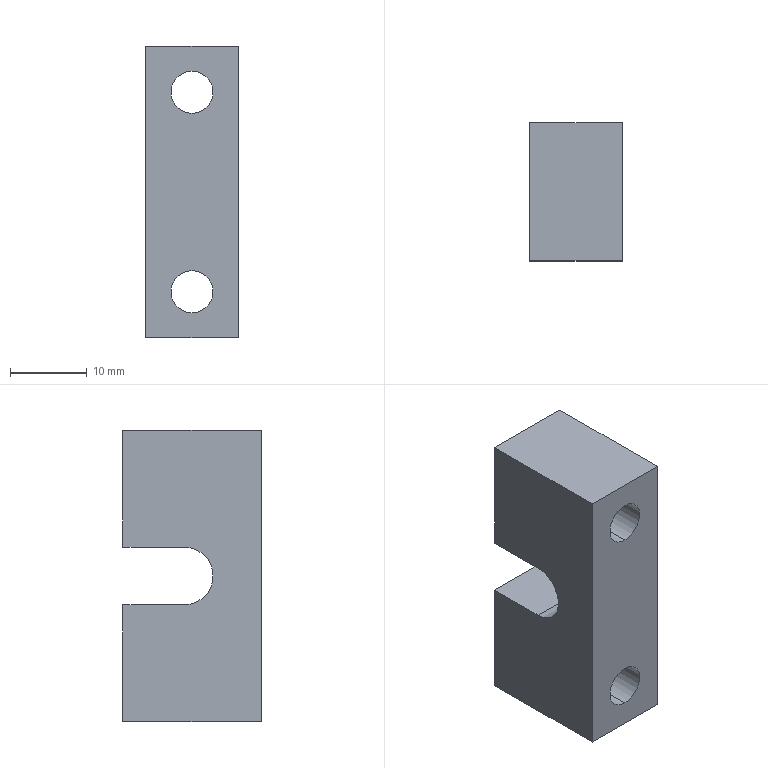Part | SolidWorks | features BaseBody 1 | 1 solid | 20 faces | box 12 x 18 x 38 mm | volume 5849 mm3 | plane 11 | cylinder 9 | commonest cylinder face diameters 5.5 x4 9.5 x4 7.5 x1
STEP:
#1=CARTESIAN_POINT('',(0.,12.5,8.25));
#2=VERTEX_POINT('',#1);
#3=CARTESIAN_POINT('',(0.,12.5,17.75));
#4=VERTEX_POINT('',#3);
#5=CARTESIAN_POINT('',(0.,12.5,13.));
#6=DIRECTION('',(0.,1.,0.));
#7=DIRECTION('',(0.,0.,1.));
#8=AXIS2_PLACEMENT_3D('',#5,#6,#7);
#9=CIRCLE('',#8,4.75);
#10=EDGE_CURVE('',#2,#4,#9,.T.);
#11=ORIENTED_EDGE('',*,*,#10,.F.);
#12=CARTESIAN_POINT('',(0.,18.,8.25));
#13=VERTEX_POINT('',#12);
#14=CARTESIAN_POINT('',(0.,18.,8.25));
#15=DIRECTION('',(0.,1.,0.));
#16=VECTOR('',#15,1000.);
#17=LINE('',#14,#16);
#18=EDGE_CURVE('',#2,#13,#17,.T.);
#19=ORIENTED_EDGE('',*,*,#18,.T.);
#20=CARTESIAN_POINT('',(0.,18.,17.75));
#21=VERTEX_POINT('',#20);
#22=CARTESIAN_POINT('',(0.,18.,13.));
#23=DIRECTION('',(0.,1.,0.));
#24=DIRECTION('',(0.,0.,1.));
#25=AXIS2_PLACEMENT_3D('',#22,#23,#24);
#26=CIRCLE('',#25,4.75);
#27=EDGE_CURVE('',#13,#21,#26,.T.);
#28=ORIENTED_EDGE('',*,*,#27,.T.);
#29=CARTESIAN_POINT('',(0.,18.,17.75));
#30=DIRECTION('',(0.,1.,0.));
#31=VECTOR('',#30,1000.);
#32=LINE('',#29,#31);
#33=EDGE_CURVE('',#4,#21,#32,.T.);
#34=ORIENTED_EDGE('',*,*,#33,.F.);
#35=EDGE_LOOP('',(#11,#19,#28,#34));
#36=FACE_OUTER_BOUND('',#35,.T.);
#37=CARTESIAN_POINT('',(0.,18.,13.));
#38=DIRECTION('',(0.,1.,0.));
#39=DIRECTION('',(0.,0.,1.));
#40=AXIS2_PLACEMENT_3D('',#37,#38,#39);
#41=CYLINDRICAL_SURFACE('',#40,4.75);
#42=ADVANCED_FACE('',(#36),#41,.F.);
#43=CARTESIAN_POINT('',(0.,12.5,-17.75));
#44=VERTEX_POINT('',#43);
#45=CARTESIAN_POINT('',(0.,12.5,-8.25));
#46=VERTEX_POINT('',#45);
#47=CARTESIAN_POINT('',(0.,12.5,-13.));
#48=DIRECTION('',(0.,1.,0.));
#49=DIRECTION('',(0.,0.,1.));
#50=AXIS2_PLACEMENT_3D('',#47,#48,#49);
#51=CIRCLE('',#50,4.75);
#52=EDGE_CURVE('',#44,#46,#51,.T.);
#53=ORIENTED_EDGE('',*,*,#52,.F.);
#54=CARTESIAN_POINT('',(0.,18.,-17.75));
#55=VERTEX_POINT('',#54);
#56=CARTESIAN_POINT('',(0.,18.,-17.75));
#57=DIRECTION('',(0.,1.,0.));
#58=VECTOR('',#57,1000.);
#59=LINE('',#56,#58);
#60=EDGE_CURVE('',#44,#55,#59,.T.);
#61=ORIENTED_EDGE('',*,*,#60,.T.);
#62=CARTESIAN_POINT('',(0.,18.,-8.25));
#63=VERTEX_POINT('',#62);
#64=CARTESIAN_POINT('',(0.,18.,-13.));
#65=DIRECTION('',(0.,1.,0.));
#66=DIRECTION('',(0.,0.,1.));
#67=AXIS2_PLACEMENT_3D('',#64,#65,#66);
#68=CIRCLE('',#67,4.75);
#69=EDGE_CURVE('',#55,#63,#68,.T.);
#70=ORIENTED_EDGE('',*,*,#69,.T.);
#71=CARTESIAN_POINT('',(0.,18.,-8.25));
#72=DIRECTION('',(0.,1.,0.));
#73=VECTOR('',#72,1000.);
#74=LINE('',#71,#73);
#75=EDGE_CURVE('',#46,#63,#74,.T.);
#76=ORIENTED_EDGE('',*,*,#75,.F.);
#77=EDGE_LOOP('',(#53,#61,#70,#76));
#78=FACE_OUTER_BOUND('',#77,.T.);
#79=CARTESIAN_POINT('',(0.,18.,-13.));
#80=DIRECTION('',(0.,1.,0.));
#81=DIRECTION('',(0.,0.,1.));
#82=AXIS2_PLACEMENT_3D('',#79,#80,#81);
#83=CYLINDRICAL_SURFACE('',#82,4.75);
#84=ADVANCED_FACE('',(#78),#83,.F.);
#85=CARTESIAN_POINT('',(0.,0.,-10.25));
#86=VERTEX_POINT('',#85);
#87=CARTESIAN_POINT('',(0.,0.,-15.75));
#88=VERTEX_POINT('',#87);
#89=CARTESIAN_POINT('',(0.,0.,-13.));
#90=DIRECTION('',(0.,-1.,0.));
#91=DIRECTION('',(0.,0.,1.));
#92=AXIS2_PLACEMENT_3D('',#89,#90,#91);
#93=CIRCLE('',#92,2.75);
#94=EDGE_CURVE('',#86,#88,#93,.T.);
#95=ORIENTED_EDGE('',*,*,#94,.T.);
#96=CARTESIAN_POINT('',(0.,12.5,-15.75));
#97=VERTEX_POINT('',#96);
#98=CARTESIAN_POINT('',(0.,18.,-15.75));
#99=DIRECTION('',(0.,1.,0.));
#100=VECTOR('',#99,1000.);
#101=LINE('',#98,#100);
#102=EDGE_CURVE('',#88,#97,#101,.T.);
#103=ORIENTED_EDGE('',*,*,#102,.T.);
#104=CARTESIAN_POINT('',(0.,12.5,-10.25));
#105=VERTEX_POINT('',#104);
#106=CARTESIAN_POINT('',(0.,12.5,-13.));
#107=DIRECTION('',(0.,-1.,0.));
#108=DIRECTION('',(0.,0.,1.));
#109=AXIS2_PLACEMENT_3D('',#106,#107,#108);
#110=CIRCLE('',#109,2.75);
#111=EDGE_CURVE('',#105,#97,#110,.T.);
#112=ORIENTED_EDGE('',*,*,#111,.F.);
#113=CARTESIAN_POINT('',(0.,18.,-10.25));
#114=DIRECTION('',(0.,1.,0.));
#115=VECTOR('',#114,1000.);
#116=LINE('',#113,#115);
#117=EDGE_CURVE('',#86,#105,#116,.T.);
#118=ORIENTED_EDGE('',*,*,#117,.F.);
#119=EDGE_LOOP('',(#95,#103,#112,#118));
#120=FACE_OUTER_BOUND('',#119,.T.);
#121=CARTESIAN_POINT('',(0.,18.,-13.));
#122=DIRECTION('',(0.,1.,0.));
#123=DIRECTION('',(0.,0.,1.));
#124=AXIS2_PLACEMENT_3D('',#121,#122,#123);
#125=CYLINDRICAL_SURFACE('',#124,2.75);
#126=ADVANCED_FACE('',(#120),#125,.F.);
#127=CARTESIAN_POINT('',(0.,0.,15.75));
#128=VERTEX_POINT('',#127);
#129=CARTESIAN_POINT('',(0.,0.,10.25));
#130=VERTEX_POINT('',#129);
#131=CARTESIAN_POINT('',(0.,0.,13.));
#132=DIRECTION('',(0.,-1.,0.));
#133=DIRECTION('',(0.,0.,1.));
#134=AXIS2_PLACEMENT_3D('',#131,#132,#133);
#135=CIRCLE('',#134,2.75);
#136=EDGE_CURVE('',#128,#130,#135,.T.);
#137=ORIENTED_EDGE('',*,*,#136,.T.);
#138=CARTESIAN_POINT('',(0.,12.5,10.25));
#139=VERTEX_POINT('',#138);
#140=CARTESIAN_POINT('',(0.,18.,10.25));
#141=DIRECTION('',(0.,1.,0.));
#142=VECTOR('',#141,1000.);
#143=LINE('',#140,#142);
#144=EDGE_CURVE('',#130,#139,#143,.T.);
#145=ORIENTED_EDGE('',*,*,#144,.T.);
#146=CARTESIAN_POINT('',(0.,12.5,15.75));
#147=VERTEX_POINT('',#146);
#148=CARTESIAN_POINT('',(0.,12.5,13.));
#149=DIRECTION('',(0.,-1.,0.));
#150=DIRECTION('',(0.,0.,1.));
#151=AXIS2_PLACEMENT_3D('',#148,#149,#150);
#152=CIRCLE('',#151,2.75);
#153=EDGE_CURVE('',#147,#139,#152,.T.);
#154=ORIENTED_EDGE('',*,*,#153,.F.);
#155=CARTESIAN_POINT('',(0.,18.,15.75));
#156=DIRECTION('',(0.,1.,0.));
#157=VECTOR('',#156,1000.);
#158=LINE('',#155,#157);
#159=EDGE_CURVE('',#128,#147,#158,.T.);
#160=ORIENTED_EDGE('',*,*,#159,.F.);
#161=EDGE_LOOP('',(#137,#145,#154,#160));
#162=FACE_OUTER_BOUND('',#161,.T.);
#163=CARTESIAN_POINT('',(0.,18.,13.));
#164=DIRECTION('',(0.,1.,0.));
#165=DIRECTION('',(0.,0.,1.));
#166=AXIS2_PLACEMENT_3D('',#163,#164,#165);
#167=CYLINDRICAL_SURFACE('',#166,2.75);
#168=ADVANCED_FACE('',(#162),#167,.F.);
#169=CARTESIAN_POINT('',(-6.,10.,3.75));
#170=VERTEX_POINT('',#169);
#171=CARTESIAN_POINT('',(-6.,18.,3.75));
#172=VERTEX_POINT('',#171);
#173=CARTESIAN_POINT('',(-6.,10.,3.75));
#174=DIRECTION('',(0.,1.,0.));
#175=VECTOR('',#174,1000.);
#176=LINE('',#173,#175);
#177=EDGE_CURVE('',#170,#172,#176,.T.);
#178=ORIENTED_EDGE('',*,*,#177,.F.);
#179=CARTESIAN_POINT('',(-6.,10.,-3.75));
#180=VERTEX_POINT('',#179);
#181=CARTESIAN_POINT('',(-6.,10.,0.));
#182=DIRECTION('',(-1.,0.,0.));
#183=DIRECTION('',(0.,0.,1.));
#184=AXIS2_PLACEMENT_3D('',#181,#182,#183);
#185=CIRCLE('',#184,3.75);
#186=EDGE_CURVE('',#180,#170,#185,.T.);
#187=ORIENTED_EDGE('',*,*,#186,.F.);
#188=CARTESIAN_POINT('',(-6.,18.,-3.75));
#189=VERTEX_POINT('',#188);
#190=CARTESIAN_POINT('',(-6.,10.,-3.75));
#191=DIRECTION('',(0.,-1.,0.));
#192=VECTOR('',#191,1000.);
#193=LINE('',#190,#192);
#194=EDGE_CURVE('',#189,#180,#193,.T.);
#195=ORIENTED_EDGE('',*,*,#194,.F.);
#196=CARTESIAN_POINT('',(-6.,18.,-19.));
#197=VERTEX_POINT('',#196);
#198=CARTESIAN_POINT('',(-6.,18.,0.));
#199=DIRECTION('',(0.,0.,1.));
#200=VECTOR('',#199,1000.);
#201=LINE('',#198,#200);
#202=EDGE_CURVE('',#197,#189,#201,.T.);
#203=ORIENTED_EDGE('',*,*,#202,.F.);
#204=CARTESIAN_POINT('',(-6.,0.,-19.));
#205=VERTEX_POINT('',#204);
#206=CARTESIAN_POINT('',(-6.,10.,-19.));
#207=DIRECTION('',(0.,1.,0.));
#208=VECTOR('',#207,1000.);
#209=LINE('',#206,#208);
#210=EDGE_CURVE('',#205,#197,#209,.T.);
#211=ORIENTED_EDGE('',*,*,#210,.F.);
#212=CARTESIAN_POINT('',(-6.,0.,19.));
#213=VERTEX_POINT('',#212);
#214=CARTESIAN_POINT('',(-6.,0.,0.));
#215=DIRECTION('',(0.,0.,-1.));
#216=VECTOR('',#215,1000.);
#217=LINE('',#214,#216);
#218=EDGE_CURVE('',#213,#205,#217,.T.);
#219=ORIENTED_EDGE('',*,*,#218,.F.);
#220=CARTESIAN_POINT('',(-6.,18.,19.));
#221=VERTEX_POINT('',#220);
#222=CARTESIAN_POINT('',(-6.,10.,19.));
#223=DIRECTION('',(0.,-1.,0.));
#224=VECTOR('',#223,1000.);
#225=LINE('',#222,#224);
#226=EDGE_CURVE('',#221,#213,#225,.T.);
#227=ORIENTED_EDGE('',*,*,#226,.F.);
#228=CARTESIAN_POINT('',(-6.,18.,0.));
#229=DIRECTION('',(0.,0.,1.));
#230=VECTOR('',#229,1000.);
#231=LINE('',#228,#230);
#232=EDGE_CURVE('',#172,#221,#231,.T.);
#233=ORIENTED_EDGE('',*,*,#232,.F.);
#234=EDGE_LOOP('',(#178,#187,#195,#203,#211,#219,#227,#233));
#235=FACE_OUTER_BOUND('',#234,.T.);
#236=CARTESIAN_POINT('',(-6.,10.,0.));
#237=DIRECTION('',(1.,0.,0.));
#238=DIRECTION('',(0.,0.,-1.));
#239=AXIS2_PLACEMENT_3D('',#236,#237,#238);
#240=PLANE('',#239);
#241=ADVANCED_FACE('',(#235),#240,.F.);
#242=CARTESIAN_POINT('',(6.,18.,19.));
#243=VERTEX_POINT('',#242);
#244=CARTESIAN_POINT('',(6.,18.,19.));
#245=DIRECTION('',(-1.,0.,0.));
#246=VECTOR('',#245,1000.);
#247=LINE('',#244,#246);
#248=EDGE_CURVE('',#243,#221,#247,.T.);
#249=ORIENTED_EDGE('',*,*,#248,.F.);
#250=CARTESIAN_POINT('',(6.,18.,3.75));
#251=VERTEX_POINT('',#250);
#252=CARTESIAN_POINT('',(6.,18.,3.75));
#253=DIRECTION('',(0.,0.,1.));
#254=VECTOR('',#253,1000.);
#255=LINE('',#252,#254);
#256=EDGE_CURVE('',#251,#243,#255,.T.);
#257=ORIENTED_EDGE('',*,*,#256,.F.);
#258=CARTESIAN_POINT('',(6.,18.,3.75));
#259=DIRECTION('',(1.,0.,0.));
#260=VECTOR('',#259,1000.);
#261=LINE('',#258,#260);
#262=EDGE_CURVE('',#172,#251,#261,.T.);
#263=ORIENTED_EDGE('',*,*,#262,.F.);
#264=ORIENTED_EDGE('',*,*,#232,.T.);
#265=EDGE_LOOP('',(#249,#257,#263,#264));
#266=FACE_OUTER_BOUND('',#265,.T.);
#267=CARTESIAN_POINT('',(0.,18.,13.));
#268=DIRECTION('',(0.,1.,0.));
#269=DIRECTION('',(0.,0.,1.));
#270=AXIS2_PLACEMENT_3D('',#267,#268,#269);
#271=CIRCLE('',#270,4.75);
#272=EDGE_CURVE('',#21,#13,#271,.T.);
#273=ORIENTED_EDGE('',*,*,#272,.F.);
#274=ORIENTED_EDGE('',*,*,#27,.F.);
#275=EDGE_LOOP('',(#273,#274));
#276=FACE_BOUND('',#275,.T.);
#277=CARTESIAN_POINT('',(6.,18.,3.75));
#278=DIRECTION('',(0.,-1.,0.));
#279=DIRECTION('',(0.,0.,-1.));
#280=AXIS2_PLACEMENT_3D('',#277,#278,#279);
#281=PLANE('',#280);
#282=ADVANCED_FACE('',(#266,#276),#281,.F.);
#283=ORIENTED_EDGE('',*,*,#262,.T.);
#284=CARTESIAN_POINT('',(6.,10.,3.75));
#285=VERTEX_POINT('',#284);
#286=CARTESIAN_POINT('',(6.,10.,3.75));
#287=DIRECTION('',(0.,1.,0.));
#288=VECTOR('',#287,1000.);
#289=LINE('',#286,#288);
#290=EDGE_CURVE('',#285,#251,#289,.T.);
#291=ORIENTED_EDGE('',*,*,#290,.F.);
#292=CARTESIAN_POINT('',(6.,10.,3.75));
#293=DIRECTION('',(1.,0.,0.));
#294=VECTOR('',#293,1000.);
#295=LINE('',#292,#294);
#296=EDGE_CURVE('',#170,#285,#295,.T.);
#297=ORIENTED_EDGE('',*,*,#296,.F.);
#298=ORIENTED_EDGE('',*,*,#177,.T.);
#299=EDGE_LOOP('',(#283,#291,#297,#298));
#300=FACE_OUTER_BOUND('',#299,.T.);
#301=CARTESIAN_POINT('',(6.,10.,3.75));
#302=DIRECTION('',(0.,0.,1.));
#303=DIRECTION('',(1.,0.,0.));
#304=AXIS2_PLACEMENT_3D('',#301,#302,#303);
#305=PLANE('',#304);
#306=ADVANCED_FACE('',(#300),#305,.F.);
#307=ORIENTED_EDGE('',*,*,#296,.T.);
#308=CARTESIAN_POINT('',(6.,10.,-3.75));
#309=VERTEX_POINT('',#308);
#310=CARTESIAN_POINT('',(6.,10.,0.));
#311=DIRECTION('',(-1.,0.,0.));
#312=DIRECTION('',(0.,0.,1.));
#313=AXIS2_PLACEMENT_3D('',#310,#311,#312);
#314=CIRCLE('',#313,3.75);
#315=EDGE_CURVE('',#309,#285,#314,.T.);
#316=ORIENTED_EDGE('',*,*,#315,.F.);
#317=CARTESIAN_POINT('',(6.,10.,-3.75));
#318=DIRECTION('',(1.,0.,0.));
#319=VECTOR('',#318,1000.);
#320=LINE('',#317,#319);
#321=EDGE_CURVE('',#180,#309,#320,.T.);
#322=ORIENTED_EDGE('',*,*,#321,.F.);
#323=ORIENTED_EDGE('',*,*,#186,.T.);
#324=EDGE_LOOP('',(#307,#316,#322,#323));
#325=FACE_OUTER_BOUND('',#324,.T.);
#326=CARTESIAN_POINT('',(6.,10.,0.));
#327=DIRECTION('',(-1.,0.,0.));
#328=DIRECTION('',(0.,0.,1.));
#329=AXIS2_PLACEMENT_3D('',#326,#327,#328);
#330=CYLINDRICAL_SURFACE('',#329,3.75);
#331=ADVANCED_FACE('',(#325),#330,.F.);
#332=ORIENTED_EDGE('',*,*,#321,.T.);
#333=CARTESIAN_POINT('',(6.,18.,-3.75));
#334=VERTEX_POINT('',#333);
#335=CARTESIAN_POINT('',(6.,18.,-3.75));
#336=DIRECTION('',(0.,-1.,0.));
#337=VECTOR('',#336,1000.);
#338=LINE('',#335,#337);
#339=EDGE_CURVE('',#334,#309,#338,.T.);
#340=ORIENTED_EDGE('',*,*,#339,.F.);
#341=CARTESIAN_POINT('',(6.,18.,-3.75));
#342=DIRECTION('',(1.,0.,0.));
#343=VECTOR('',#342,1000.);
#344=LINE('',#341,#343);
#345=EDGE_CURVE('',#189,#334,#344,.T.);
#346=ORIENTED_EDGE('',*,*,#345,.F.);
#347=ORIENTED_EDGE('',*,*,#194,.T.);
#348=EDGE_LOOP('',(#332,#340,#346,#347));
#349=FACE_OUTER_BOUND('',#348,.T.);
#350=CARTESIAN_POINT('',(6.,18.,-3.75));
#351=DIRECTION('',(0.,0.,-1.));
#352=DIRECTION('',(-1.,0.,0.));
#353=AXIS2_PLACEMENT_3D('',#350,#351,#352);
#354=PLANE('',#353);
#355=ADVANCED_FACE('',(#349),#354,.F.);
#356=ORIENTED_EDGE('',*,*,#345,.T.);
#357=CARTESIAN_POINT('',(6.,18.,-19.));
#358=VERTEX_POINT('',#357);
#359=CARTESIAN_POINT('',(6.,18.,-19.));
#360=DIRECTION('',(0.,0.,1.));
#361=VECTOR('',#360,1000.);
#362=LINE('',#359,#361);
#363=EDGE_CURVE('',#358,#334,#362,.T.);
#364=ORIENTED_EDGE('',*,*,#363,.F.);
#365=CARTESIAN_POINT('',(6.,18.,-19.));
#366=DIRECTION('',(1.,0.,0.));
#367=VECTOR('',#366,1000.);
#368=LINE('',#365,#367);
#369=EDGE_CURVE('',#197,#358,#368,.T.);
#370=ORIENTED_EDGE('',*,*,#369,.F.);
#371=ORIENTED_EDGE('',*,*,#202,.T.);
#372=EDGE_LOOP('',(#356,#364,#370,#371));
#373=FACE_OUTER_BOUND('',#372,.T.);
#374=CARTESIAN_POINT('',(0.,18.,-13.));
#375=DIRECTION('',(0.,1.,0.));
#376=DIRECTION('',(0.,0.,1.));
#377=AXIS2_PLACEMENT_3D('',#374,#375,#376);
#378=CIRCLE('',#377,4.75);
#379=EDGE_CURVE('',#63,#55,#378,.T.);
#380=ORIENTED_EDGE('',*,*,#379,.F.);
#381=ORIENTED_EDGE('',*,*,#69,.F.);
#382=EDGE_LOOP('',(#380,#381));
#383=FACE_BOUND('',#382,.T.);
#384=CARTESIAN_POINT('',(6.,18.,-19.));
#385=DIRECTION('',(0.,-1.,0.));
#386=DIRECTION('',(0.,0.,-1.));
#387=AXIS2_PLACEMENT_3D('',#384,#385,#386);
#388=PLANE('',#387);
#389=ADVANCED_FACE('',(#373,#383),#388,.F.);
#390=ORIENTED_EDGE('',*,*,#369,.T.);
#391=CARTESIAN_POINT('',(6.,0.,-19.));
#392=VERTEX_POINT('',#391);
#393=CARTESIAN_POINT('',(6.,0.,-19.));
#394=DIRECTION('',(0.,1.,0.));
#395=VECTOR('',#394,1000.);
#396=LINE('',#393,#395);
#397=EDGE_CURVE('',#392,#358,#396,.T.);
#398=ORIENTED_EDGE('',*,*,#397,.F.);
#399=CARTESIAN_POINT('',(6.,0.,-19.));
#400=DIRECTION('',(1.,0.,0.));
#401=VECTOR('',#400,1000.);
#402=LINE('',#399,#401);
#403=EDGE_CURVE('',#205,#392,#402,.T.);
#404=ORIENTED_EDGE('',*,*,#403,.F.);
#405=ORIENTED_EDGE('',*,*,#210,.T.);
#406=EDGE_LOOP('',(#390,#398,#404,#405));
#407=FACE_OUTER_BOUND('',#406,.T.);
#408=CARTESIAN_POINT('',(6.,0.,-19.));
#409=DIRECTION('',(0.,0.,1.));
#410=DIRECTION('',(1.,0.,0.));
#411=AXIS2_PLACEMENT_3D('',#408,#409,#410);
#412=PLANE('',#411);
#413=ADVANCED_FACE('',(#407),#412,.F.);
#414=ORIENTED_EDGE('',*,*,#403,.T.);
#415=CARTESIAN_POINT('',(6.,0.,19.));
#416=VERTEX_POINT('',#415);
#417=CARTESIAN_POINT('',(6.,0.,19.));
#418=DIRECTION('',(0.,0.,-1.));
#419=VECTOR('',#418,1000.);
#420=LINE('',#417,#419);
#421=EDGE_CURVE('',#416,#392,#420,.T.);
#422=ORIENTED_EDGE('',*,*,#421,.F.);
#423=CARTESIAN_POINT('',(6.,0.,19.));
#424=DIRECTION('',(1.,0.,0.));
#425=VECTOR('',#424,1000.);
#426=LINE('',#423,#425);
#427=EDGE_CURVE('',#213,#416,#426,.T.);
#428=ORIENTED_EDGE('',*,*,#427,.F.);
#429=ORIENTED_EDGE('',*,*,#218,.T.);
#430=EDGE_LOOP('',(#414,#422,#428,#429));
#431=FACE_OUTER_BOUND('',#430,.T.);
#432=ORIENTED_EDGE('',*,*,#94,.F.);
#433=CARTESIAN_POINT('',(0.,0.,-13.));
#434=DIRECTION('',(0.,-1.,0.));
#435=DIRECTION('',(0.,0.,1.));
#436=AXIS2_PLACEMENT_3D('',#433,#434,#435);
#437=CIRCLE('',#436,2.75);
#438=EDGE_CURVE('',#88,#86,#437,.T.);
#439=ORIENTED_EDGE('',*,*,#438,.F.);
#440=EDGE_LOOP('',(#432,#439));
#441=FACE_BOUND('',#440,.T.);
#442=ORIENTED_EDGE('',*,*,#136,.F.);
#443=CARTESIAN_POINT('',(0.,0.,13.));
#444=DIRECTION('',(0.,-1.,0.));
#445=DIRECTION('',(0.,0.,1.));
#446=AXIS2_PLACEMENT_3D('',#443,#444,#445);
#447=CIRCLE('',#446,2.75);
#448=EDGE_CURVE('',#130,#128,#447,.T.);
#449=ORIENTED_EDGE('',*,*,#448,.F.);
#450=EDGE_LOOP('',(#442,#449));
#451=FACE_BOUND('',#450,.T.);
#452=CARTESIAN_POINT('',(6.,0.,19.));
#453=DIRECTION('',(0.,1.,0.));
#454=DIRECTION('',(0.,0.,1.));
#455=AXIS2_PLACEMENT_3D('',#452,#453,#454);
#456=PLANE('',#455);
#457=ADVANCED_FACE('',(#431,#441,#451),#456,.F.);
#458=ORIENTED_EDGE('',*,*,#427,.T.);
#459=CARTESIAN_POINT('',(6.,18.,19.));
#460=DIRECTION('',(0.,-1.,0.));
#461=VECTOR('',#460,1000.);
#462=LINE('',#459,#461);
#463=EDGE_CURVE('',#243,#416,#462,.T.);
#464=ORIENTED_EDGE('',*,*,#463,.F.);
#465=ORIENTED_EDGE('',*,*,#248,.T.);
#466=ORIENTED_EDGE('',*,*,#226,.T.);
#467=EDGE_LOOP('',(#458,#464,#465,#466));
#468=FACE_OUTER_BOUND('',#467,.T.);
#469=CARTESIAN_POINT('',(6.,18.,19.));
#470=DIRECTION('',(0.,0.,-1.));
#471=DIRECTION('',(-1.,0.,0.));
#472=AXIS2_PLACEMENT_3D('',#469,#470,#471);
#473=PLANE('',#472);
#474=ADVANCED_FACE('',(#468),#473,.F.);
#475=ORIENTED_EDGE('',*,*,#315,.T.);
#476=ORIENTED_EDGE('',*,*,#290,.T.);
#477=ORIENTED_EDGE('',*,*,#256,.T.);
#478=ORIENTED_EDGE('',*,*,#463,.T.);
#479=ORIENTED_EDGE('',*,*,#421,.T.);
#480=ORIENTED_EDGE('',*,*,#397,.T.);
#481=ORIENTED_EDGE('',*,*,#363,.T.);
#482=ORIENTED_EDGE('',*,*,#339,.T.);
#483=EDGE_LOOP('',(#475,#476,#477,#478,#479,#480,#481,#482));
#484=FACE_OUTER_BOUND('',#483,.T.);
#485=CARTESIAN_POINT('',(6.,10.,0.));
#486=DIRECTION('',(1.,0.,0.));
#487=DIRECTION('',(0.,0.,-1.));
#488=AXIS2_PLACEMENT_3D('',#485,#486,#487);
#489=PLANE('',#488);
#490=ADVANCED_FACE('',(#484),#489,.T.);
#491=ORIENTED_EDGE('',*,*,#18,.F.);
#492=CARTESIAN_POINT('',(0.,12.5,13.));
#493=DIRECTION('',(0.,1.,0.));
#494=DIRECTION('',(0.,0.,1.));
#495=AXIS2_PLACEMENT_3D('',#492,#493,#494);
#496=CIRCLE('',#495,4.75);
#497=EDGE_CURVE('',#4,#2,#496,.T.);
#498=ORIENTED_EDGE('',*,*,#497,.F.);
#499=ORIENTED_EDGE('',*,*,#33,.T.);
#500=ORIENTED_EDGE('',*,*,#272,.T.);
#501=EDGE_LOOP('',(#491,#498,#499,#500));
#502=FACE_OUTER_BOUND('',#501,.T.);
#503=CARTESIAN_POINT('',(0.,18.,13.));
#504=DIRECTION('',(0.,1.,0.));
#505=DIRECTION('',(0.,0.,1.));
#506=AXIS2_PLACEMENT_3D('',#503,#504,#505);
#507=CYLINDRICAL_SURFACE('',#506,4.75);
#508=ADVANCED_FACE('',(#502),#507,.F.);
#509=ORIENTED_EDGE('',*,*,#60,.F.);
#510=CARTESIAN_POINT('',(0.,12.5,-13.));
#511=DIRECTION('',(0.,1.,0.));
#512=DIRECTION('',(0.,0.,1.));
#513=AXIS2_PLACEMENT_3D('',#510,#511,#512);
#514=CIRCLE('',#513,4.75);
#515=EDGE_CURVE('',#46,#44,#514,.T.);
#516=ORIENTED_EDGE('',*,*,#515,.F.);
#517=ORIENTED_EDGE('',*,*,#75,.T.);
#518=ORIENTED_EDGE('',*,*,#379,.T.);
#519=EDGE_LOOP('',(#509,#516,#517,#518));
#520=FACE_OUTER_BOUND('',#519,.T.);
#521=CARTESIAN_POINT('',(0.,18.,-13.));
#522=DIRECTION('',(0.,1.,0.));
#523=DIRECTION('',(0.,0.,1.));
#524=AXIS2_PLACEMENT_3D('',#521,#522,#523);
#525=CYLINDRICAL_SURFACE('',#524,4.75);
#526=ADVANCED_FACE('',(#520),#525,.F.);
#527=ORIENTED_EDGE('',*,*,#102,.F.);
#528=ORIENTED_EDGE('',*,*,#438,.T.);
#529=ORIENTED_EDGE('',*,*,#117,.T.);
#530=CARTESIAN_POINT('',(0.,12.5,-13.));
#531=DIRECTION('',(0.,-1.,0.));
#532=DIRECTION('',(0.,0.,1.));
#533=AXIS2_PLACEMENT_3D('',#530,#531,#532);
#534=CIRCLE('',#533,2.75);
#535=EDGE_CURVE('',#97,#105,#534,.T.);
#536=ORIENTED_EDGE('',*,*,#535,.F.);
#537=EDGE_LOOP('',(#527,#528,#529,#536));
#538=FACE_OUTER_BOUND('',#537,.T.);
#539=CARTESIAN_POINT('',(0.,18.,-13.));
#540=DIRECTION('',(0.,1.,0.));
#541=DIRECTION('',(0.,0.,1.));
#542=AXIS2_PLACEMENT_3D('',#539,#540,#541);
#543=CYLINDRICAL_SURFACE('',#542,2.75);
#544=ADVANCED_FACE('',(#538),#543,.F.);
#545=ORIENTED_EDGE('',*,*,#144,.F.);
#546=ORIENTED_EDGE('',*,*,#448,.T.);
#547=ORIENTED_EDGE('',*,*,#159,.T.);
#548=CARTESIAN_POINT('',(0.,12.5,13.));
#549=DIRECTION('',(0.,-1.,0.));
#550=DIRECTION('',(0.,0.,1.));
#551=AXIS2_PLACEMENT_3D('',#548,#549,#550);
#552=CIRCLE('',#551,2.75);
#553=EDGE_CURVE('',#139,#147,#552,.T.);
#554=ORIENTED_EDGE('',*,*,#553,.F.);
#555=EDGE_LOOP('',(#545,#546,#547,#554));
#556=FACE_OUTER_BOUND('',#555,.T.);
#557=CARTESIAN_POINT('',(0.,18.,13.));
#558=DIRECTION('',(0.,1.,0.));
#559=DIRECTION('',(0.,0.,1.));
#560=AXIS2_PLACEMENT_3D('',#557,#558,#559);
#561=CYLINDRICAL_SURFACE('',#560,2.75);
#562=ADVANCED_FACE('',(#556),#561,.F.);
#563=ORIENTED_EDGE('',*,*,#153,.T.);
#564=ORIENTED_EDGE('',*,*,#553,.T.);
#565=EDGE_LOOP('',(#563,#564));
#566=FACE_BOUND('',#565,.T.);
#567=ORIENTED_EDGE('',*,*,#497,.T.);
#568=ORIENTED_EDGE('',*,*,#10,.T.);
#569=EDGE_LOOP('',(#567,#568));
#570=FACE_OUTER_BOUND('',#569,.T.);
#571=CARTESIAN_POINT('',(0.,12.5,15.75));
#572=DIRECTION('',(0.,1.,0.));
#573=DIRECTION('',(0.,0.,1.));
#574=AXIS2_PLACEMENT_3D('',#571,#572,#573);
#575=PLANE('',#574);
#576=ADVANCED_FACE('',(#566,#570),#575,.T.);
#577=ORIENTED_EDGE('',*,*,#111,.T.);
#578=ORIENTED_EDGE('',*,*,#535,.T.);
#579=EDGE_LOOP('',(#577,#578));
#580=FACE_BOUND('',#579,.T.);
#581=ORIENTED_EDGE('',*,*,#515,.T.);
#582=ORIENTED_EDGE('',*,*,#52,.T.);
#583=EDGE_LOOP('',(#581,#582));
#584=FACE_OUTER_BOUND('',#583,.T.);
#585=CARTESIAN_POINT('',(0.,12.5,-10.25));
#586=DIRECTION('',(0.,1.,0.));
#587=DIRECTION('',(0.,0.,1.));
#588=AXIS2_PLACEMENT_3D('',#585,#586,#587);
#589=PLANE('',#588);
#590=ADVANCED_FACE('',(#580,#584),#589,.T.);
#591=CLOSED_SHELL('',(#42,#84,#126,#168,#241,#282,#306,#331,#355,#389,#413,#457,#474,#490,#508,#526,#544,#562,#576,#590));
#592=MANIFOLD_SOLID_BREP('',#591);
#593=CARTESIAN_POINT('',(0.,0.,0.));
#594=DIRECTION('',(0.,0.,1.));
#595=DIRECTION('',(1.,0.,0.));
#596=AXIS2_PLACEMENT_3D('',#593,#594,#595);
#597=(LENGTH_UNIT()NAMED_UNIT(*)SI_UNIT(.MILLI.,.METRE.));
#598=UNCERTAINTY_MEASURE_WITH_UNIT(LENGTH_MEASURE(0.00001),#597,'','');
#599=(NAMED_UNIT(*)PLANE_ANGLE_UNIT()SI_UNIT($,.RADIAN.));
#600=(NAMED_UNIT(*)SI_UNIT($,.STERADIAN.)SOLID_ANGLE_UNIT());
#601=(GEOMETRIC_REPRESENTATION_CONTEXT(3)GLOBAL_UNCERTAINTY_ASSIGNED_CONTEXT((#598))GLOBAL_UNIT_ASSIGNED_CONTEXT((#597,#599,#600))REPRESENTATION_CONTEXT('',''));
#602=ADVANCED_BREP_SHAPE_REPRESENTATION('',(#592,#596),#601);